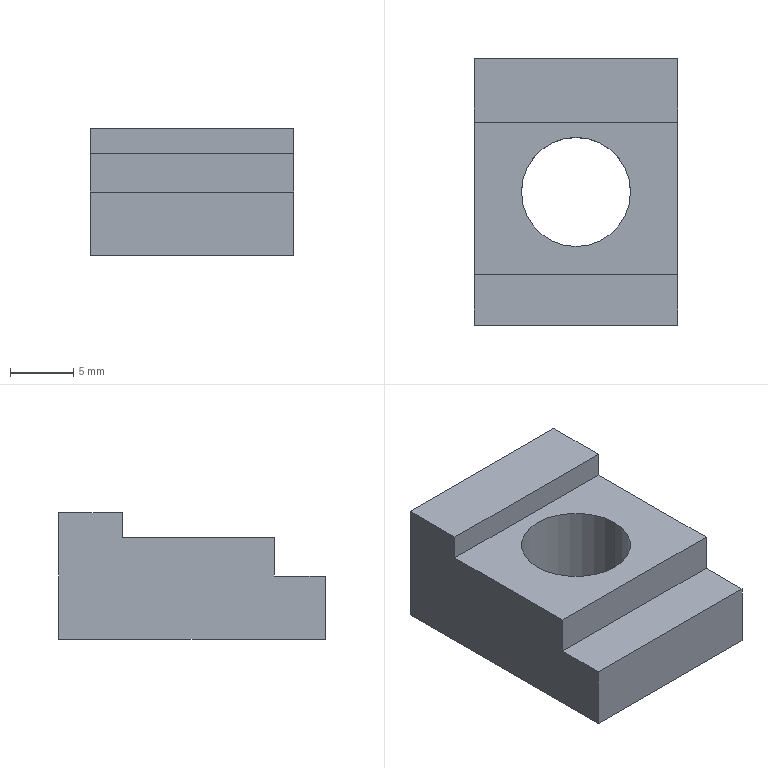Part | STEP file | 1_id1346_x_t | 1 solid | 12 faces | box 16 x 21 x 10 mm | volume 2191 mm3 | plane 10 | cylinder 2 | commonest cylinder face diameters 8.6 x2
STEP:
#1=CARTESIAN_POINT('',(0.,0.,0.));
#2=DIRECTION('',(0.,0.,1.));
#3=DIRECTION('',(1.,0.,0.));
#4=AXIS2_PLACEMENT_3D('',#1,#2,#3);
#5=CARTESIAN_POINT('',(954.138,544.1,90.11));
#6=VERTEX_POINT('',#5);
#7=CARTESIAN_POINT('',(938.138,544.1,90.11));
#8=VERTEX_POINT('',#7);
#9=CARTESIAN_POINT('',(954.138,544.1,90.11));
#10=DIRECTION('',(-1.,0.,0.));
#11=VECTOR('',#10,1.);
#12=LINE('',#9,#11);
#13=CARTESIAN_POINT('',(954.138,544.1,90.11));
#14=DIRECTION('',(0.,0.,-1.));
#15=DIRECTION('',(0.766,-0.6428,0.));
#16=AXIS2_PLACEMENT_3D('',#13,#14,#15);
#17=PLANE('',#16);
#18=CARTESIAN_POINT('',(0.,0.));
#19=DIRECTION('',(-0.766,0.6428));
#20=VECTOR('',#19,1.);
#21=LINE('',#18,#20);
#22=(GEOMETRIC_REPRESENTATION_CONTEXT(2)PARAMETRIC_REPRESENTATION_CONTEXT()REPRESENTATION_CONTEXT('',''));
#23=DEFINITIONAL_REPRESENTATION('',(#21),#22);
#24=PCURVE('',#17,#23);
#25=CARTESIAN_POINT('',(954.138,544.1,85.11));
#26=DIRECTION('',(0.,1.,0.));
#27=DIRECTION('',(0.,0.,1.));
#28=AXIS2_PLACEMENT_3D('',#25,#26,#27);
#29=PLANE('',#28);
#30=CARTESIAN_POINT('',(5.,0.));
#31=DIRECTION('',(0.,-1.));
#32=VECTOR('',#31,1.);
#33=LINE('',#30,#32);
#34=(GEOMETRIC_REPRESENTATION_CONTEXT(2)PARAMETRIC_REPRESENTATION_CONTEXT()REPRESENTATION_CONTEXT('',''));
#35=DEFINITIONAL_REPRESENTATION('',(#33),#34);
#36=PCURVE('',#29,#35);
#37=SURFACE_CURVE('',#12,(#24,#36),.PCURVE_S1.);
#38=EDGE_CURVE('',#6,#8,#37,.T.);
#39=ORIENTED_EDGE('',*,*,#38,.T.);
#40=CARTESIAN_POINT('',(938.138,539.1,90.11));
#41=VERTEX_POINT('',#40);
#42=CARTESIAN_POINT('',(938.138,544.1,90.11));
#43=DIRECTION('',(0.,-1.,0.));
#44=VECTOR('',#43,1.);
#45=LINE('',#42,#44);
#46=CARTESIAN_POINT('',(-12.257,10.285));
#47=DIRECTION('',(0.6428,0.766));
#48=VECTOR('',#47,1.);
#49=LINE('',#46,#48);
#50=(GEOMETRIC_REPRESENTATION_CONTEXT(2)PARAMETRIC_REPRESENTATION_CONTEXT()REPRESENTATION_CONTEXT('',''));
#51=DEFINITIONAL_REPRESENTATION('',(#49),#50);
#52=PCURVE('',#17,#51);
#53=CARTESIAN_POINT('',(938.138,544.1,85.11));
#54=DIRECTION('',(-1.,0.,0.));
#55=DIRECTION('',(0.,1.,0.));
#56=AXIS2_PLACEMENT_3D('',#53,#54,#55);
#57=PLANE('',#56);
#58=CARTESIAN_POINT('',(0.,-5.));
#59=DIRECTION('',(-1.,0.));
#60=VECTOR('',#59,1.);
#61=LINE('',#58,#60);
#62=(GEOMETRIC_REPRESENTATION_CONTEXT(2)PARAMETRIC_REPRESENTATION_CONTEXT()REPRESENTATION_CONTEXT('',''));
#63=DEFINITIONAL_REPRESENTATION('',(#61),#62);
#64=PCURVE('',#57,#63);
#65=SURFACE_CURVE('',#45,(#52,#64),.PCURVE_S1.);
#66=EDGE_CURVE('',#8,#41,#65,.T.);
#67=ORIENTED_EDGE('',*,*,#66,.T.);
#68=CARTESIAN_POINT('',(954.138,539.1,90.11));
#69=VERTEX_POINT('',#68);
#70=CARTESIAN_POINT('',(938.138,539.1,90.11));
#71=DIRECTION('',(1.,0.,0.));
#72=VECTOR('',#71,1.);
#73=LINE('',#70,#72);
#74=CARTESIAN_POINT('',(-9.043,14.115));
#75=DIRECTION('',(0.766,-0.6428));
#76=VECTOR('',#75,1.);
#77=LINE('',#74,#76);
#78=(GEOMETRIC_REPRESENTATION_CONTEXT(2)PARAMETRIC_REPRESENTATION_CONTEXT()REPRESENTATION_CONTEXT('',''));
#79=DEFINITIONAL_REPRESENTATION('',(#77),#78);
#80=PCURVE('',#17,#79);
#81=CARTESIAN_POINT('',(938.138,539.1,91.11));
#82=DIRECTION('',(0.,-1.,0.));
#83=DIRECTION('',(0.,0.,-1.));
#84=AXIS2_PLACEMENT_3D('',#81,#82,#83);
#85=PLANE('',#84);
#86=CARTESIAN_POINT('',(1.,0.));
#87=DIRECTION('',(0.,1.));
#88=VECTOR('',#87,1.);
#89=LINE('',#86,#88);
#90=(GEOMETRIC_REPRESENTATION_CONTEXT(2)PARAMETRIC_REPRESENTATION_CONTEXT()REPRESENTATION_CONTEXT('',''));
#91=DEFINITIONAL_REPRESENTATION('',(#89),#90);
#92=PCURVE('',#85,#91);
#93=SURFACE_CURVE('',#73,(#80,#92),.PCURVE_S1.);
#94=EDGE_CURVE('',#41,#69,#93,.T.);
#95=ORIENTED_EDGE('',*,*,#94,.T.);
#96=CARTESIAN_POINT('',(954.138,539.1,90.11));
#97=DIRECTION('',(0.,1.,0.));
#98=VECTOR('',#97,1.);
#99=LINE('',#96,#98);
#100=CARTESIAN_POINT('',(3.214,3.83));
#101=DIRECTION('',(-0.6428,-0.766));
#102=VECTOR('',#101,1.);
#103=LINE('',#100,#102);
#104=(GEOMETRIC_REPRESENTATION_CONTEXT(2)PARAMETRIC_REPRESENTATION_CONTEXT()REPRESENTATION_CONTEXT('',''));
#105=DEFINITIONAL_REPRESENTATION('',(#103),#104);
#106=PCURVE('',#17,#105);
#107=CARTESIAN_POINT('',(954.138,523.1,85.11));
#108=DIRECTION('',(1.,0.,0.));
#109=DIRECTION('',(0.,0.,1.));
#110=AXIS2_PLACEMENT_3D('',#107,#108,#109);
#111=PLANE('',#110);
#112=CARTESIAN_POINT('',(5.,-16.));
#113=DIRECTION('',(0.,-1.));
#114=VECTOR('',#113,1.);
#115=LINE('',#112,#114);
#116=(GEOMETRIC_REPRESENTATION_CONTEXT(2)PARAMETRIC_REPRESENTATION_CONTEXT()REPRESENTATION_CONTEXT('',''));
#117=DEFINITIONAL_REPRESENTATION('',(#115),#116);
#118=PCURVE('',#111,#117);
#119=SURFACE_CURVE('',#99,(#106,#118),.PCURVE_S1.);
#120=EDGE_CURVE('',#69,#6,#119,.T.);
#121=ORIENTED_EDGE('',*,*,#120,.T.);
#122=EDGE_LOOP('',(#39,#67,#95,#121));
#123=FACE_BOUND('',#122,.T.);
#124=ADVANCED_FACE('',(#123),#17,.F.);
#125=CARTESIAN_POINT('',(954.138,527.1,85.11));
#126=VERTEX_POINT('',#125);
#127=CARTESIAN_POINT('',(954.138,527.1,88.11));
#128=VERTEX_POINT('',#127);
#129=CARTESIAN_POINT('',(954.138,527.1,85.11));
#130=DIRECTION('',(0.,0.,1.));
#131=VECTOR('',#130,1.);
#132=LINE('',#129,#131);
#133=CARTESIAN_POINT('',(0.,-4.));
#134=DIRECTION('',(1.,0.));
#135=VECTOR('',#134,1.);
#136=LINE('',#133,#135);
#137=(GEOMETRIC_REPRESENTATION_CONTEXT(2)PARAMETRIC_REPRESENTATION_CONTEXT()REPRESENTATION_CONTEXT('',''));
#138=DEFINITIONAL_REPRESENTATION('',(#136),#137);
#139=PCURVE('',#111,#138);
#140=CARTESIAN_POINT('',(938.138,527.1,88.11));
#141=DIRECTION('',(0.,-1.,0.));
#142=DIRECTION('',(0.,0.,-1.));
#143=AXIS2_PLACEMENT_3D('',#140,#141,#142);
#144=PLANE('',#143);
#145=CARTESIAN_POINT('',(3.,16.));
#146=DIRECTION('',(-1.,0.));
#147=VECTOR('',#146,1.);
#148=LINE('',#145,#147);
#149=(GEOMETRIC_REPRESENTATION_CONTEXT(2)PARAMETRIC_REPRESENTATION_CONTEXT()REPRESENTATION_CONTEXT('',''));
#150=DEFINITIONAL_REPRESENTATION('',(#148),#149);
#151=PCURVE('',#144,#150);
#152=SURFACE_CURVE('',#132,(#139,#151),.PCURVE_S1.);
#153=EDGE_CURVE('',#126,#128,#152,.T.);
#154=ORIENTED_EDGE('',*,*,#153,.F.);
#155=CARTESIAN_POINT('',(954.138,523.1,85.11));
#156=VERTEX_POINT('',#155);
#157=CARTESIAN_POINT('',(954.138,523.1,85.11));
#158=DIRECTION('',(0.,1.,0.));
#159=VECTOR('',#158,1.);
#160=LINE('',#157,#159);
#161=CARTESIAN_POINT('',(0.,0.));
#162=DIRECTION('',(0.,-1.));
#163=VECTOR('',#162,1.);
#164=LINE('',#161,#163);
#165=(GEOMETRIC_REPRESENTATION_CONTEXT(2)PARAMETRIC_REPRESENTATION_CONTEXT()REPRESENTATION_CONTEXT('',''));
#166=DEFINITIONAL_REPRESENTATION('',(#164),#165);
#167=PCURVE('',#111,#166);
#168=CARTESIAN_POINT('',(938.138,523.1,85.11));
#169=DIRECTION('',(0.,0.,-1.));
#170=DIRECTION('',(0.766,-0.6428,0.));
#171=AXIS2_PLACEMENT_3D('',#168,#169,#170);
#172=PLANE('',#171);
#173=CARTESIAN_POINT('',(12.257,-10.285));
#174=DIRECTION('',(-0.6428,-0.766));
#175=VECTOR('',#174,1.);
#176=LINE('',#173,#175);
#177=(GEOMETRIC_REPRESENTATION_CONTEXT(2)PARAMETRIC_REPRESENTATION_CONTEXT()REPRESENTATION_CONTEXT('',''));
#178=DEFINITIONAL_REPRESENTATION('',(#176),#177);
#179=PCURVE('',#172,#178);
#180=SURFACE_CURVE('',#160,(#167,#179),.PCURVE_S1.);
#181=EDGE_CURVE('',#156,#126,#180,.T.);
#182=ORIENTED_EDGE('',*,*,#181,.F.);
#183=CARTESIAN_POINT('',(954.138,523.1,80.11));
#184=VERTEX_POINT('',#183);
#185=CARTESIAN_POINT('',(954.138,523.1,80.11));
#186=DIRECTION('',(0.,0.,1.));
#187=VECTOR('',#186,1.);
#188=LINE('',#185,#187);
#189=CARTESIAN_POINT('',(-5.,0.));
#190=DIRECTION('',(1.,0.));
#191=VECTOR('',#190,1.);
#192=LINE('',#189,#191);
#193=(GEOMETRIC_REPRESENTATION_CONTEXT(2)PARAMETRIC_REPRESENTATION_CONTEXT()REPRESENTATION_CONTEXT('',''));
#194=DEFINITIONAL_REPRESENTATION('',(#192),#193);
#195=PCURVE('',#111,#194);
#196=CARTESIAN_POINT('',(938.138,523.1,85.11));
#197=DIRECTION('',(0.,-1.,0.));
#198=DIRECTION('',(0.,0.,-1.));
#199=AXIS2_PLACEMENT_3D('',#196,#197,#198);
#200=PLANE('',#199);
#201=CARTESIAN_POINT('',(5.,16.));
#202=DIRECTION('',(-1.,0.));
#203=VECTOR('',#202,1.);
#204=LINE('',#201,#203);
#205=(GEOMETRIC_REPRESENTATION_CONTEXT(2)PARAMETRIC_REPRESENTATION_CONTEXT()REPRESENTATION_CONTEXT('',''));
#206=DEFINITIONAL_REPRESENTATION('',(#204),#205);
#207=PCURVE('',#200,#206);
#208=SURFACE_CURVE('',#188,(#195,#207),.PCURVE_S1.);
#209=EDGE_CURVE('',#184,#156,#208,.T.);
#210=ORIENTED_EDGE('',*,*,#209,.F.);
#211=CARTESIAN_POINT('',(954.138,544.1,80.11));
#212=VERTEX_POINT('',#211);
#213=CARTESIAN_POINT('',(954.138,544.1,80.11));
#214=DIRECTION('',(0.,-1.,0.));
#215=VECTOR('',#214,1.);
#216=LINE('',#213,#215);
#217=CARTESIAN_POINT('',(-5.,-21.));
#218=DIRECTION('',(0.,1.));
#219=VECTOR('',#218,1.);
#220=LINE('',#217,#219);
#221=(GEOMETRIC_REPRESENTATION_CONTEXT(2)PARAMETRIC_REPRESENTATION_CONTEXT()REPRESENTATION_CONTEXT('',''));
#222=DEFINITIONAL_REPRESENTATION('',(#220),#221);
#223=PCURVE('',#111,#222);
#224=CARTESIAN_POINT('',(938.138,523.1,80.11));
#225=DIRECTION('',(0.,0.,-1.));
#226=DIRECTION('',(0.766,-0.6428,0.));
#227=AXIS2_PLACEMENT_3D('',#224,#225,#226);
#228=PLANE('',#227);
#229=CARTESIAN_POINT('',(-1.242,-26.372));
#230=DIRECTION('',(0.6428,0.766));
#231=VECTOR('',#230,1.);
#232=LINE('',#229,#231);
#233=(GEOMETRIC_REPRESENTATION_CONTEXT(2)PARAMETRIC_REPRESENTATION_CONTEXT()REPRESENTATION_CONTEXT('',''));
#234=DEFINITIONAL_REPRESENTATION('',(#232),#233);
#235=PCURVE('',#228,#234);
#236=SURFACE_CURVE('',#216,(#223,#235),.PCURVE_S1.);
#237=EDGE_CURVE('',#212,#184,#236,.T.);
#238=ORIENTED_EDGE('',*,*,#237,.F.);
#239=CARTESIAN_POINT('',(954.138,544.1,80.11));
#240=DIRECTION('',(0.,0.,1.));
#241=VECTOR('',#240,1.);
#242=LINE('',#239,#241);
#243=CARTESIAN_POINT('',(-5.,-21.));
#244=DIRECTION('',(1.,0.));
#245=VECTOR('',#244,1.);
#246=LINE('',#243,#245);
#247=(GEOMETRIC_REPRESENTATION_CONTEXT(2)PARAMETRIC_REPRESENTATION_CONTEXT()REPRESENTATION_CONTEXT('',''));
#248=DEFINITIONAL_REPRESENTATION('',(#246),#247);
#249=PCURVE('',#111,#248);
#250=CARTESIAN_POINT('',(-5.,0.));
#251=DIRECTION('',(1.,0.));
#252=VECTOR('',#251,1.);
#253=LINE('',#250,#252);
#254=(GEOMETRIC_REPRESENTATION_CONTEXT(2)PARAMETRIC_REPRESENTATION_CONTEXT()REPRESENTATION_CONTEXT('',''));
#255=DEFINITIONAL_REPRESENTATION('',(#253),#254);
#256=PCURVE('',#29,#255);
#257=SURFACE_CURVE('',#242,(#249,#256),.PCURVE_S1.);
#258=EDGE_CURVE('',#212,#6,#257,.T.);
#259=ORIENTED_EDGE('',*,*,#258,.T.);
#260=ORIENTED_EDGE('',*,*,#120,.F.);
#261=CARTESIAN_POINT('',(954.138,539.1,88.11));
#262=VERTEX_POINT('',#261);
#263=CARTESIAN_POINT('',(954.138,539.1,88.11));
#264=DIRECTION('',(0.,0.,1.));
#265=VECTOR('',#264,1.);
#266=LINE('',#263,#265);
#267=CARTESIAN_POINT('',(3.,-16.));
#268=DIRECTION('',(1.,0.));
#269=VECTOR('',#268,1.);
#270=LINE('',#267,#269);
#271=(GEOMETRIC_REPRESENTATION_CONTEXT(2)PARAMETRIC_REPRESENTATION_CONTEXT()REPRESENTATION_CONTEXT('',''));
#272=DEFINITIONAL_REPRESENTATION('',(#270),#271);
#273=PCURVE('',#111,#272);
#274=CARTESIAN_POINT('',(3.,16.));
#275=DIRECTION('',(-1.,0.));
#276=VECTOR('',#275,1.);
#277=LINE('',#274,#276);
#278=(GEOMETRIC_REPRESENTATION_CONTEXT(2)PARAMETRIC_REPRESENTATION_CONTEXT()REPRESENTATION_CONTEXT('',''));
#279=DEFINITIONAL_REPRESENTATION('',(#277),#278);
#280=PCURVE('',#85,#279);
#281=SURFACE_CURVE('',#266,(#273,#280),.PCURVE_S1.);
#282=EDGE_CURVE('',#262,#69,#281,.T.);
#283=ORIENTED_EDGE('',*,*,#282,.F.);
#284=CARTESIAN_POINT('',(954.138,527.1,88.11));
#285=DIRECTION('',(0.,1.,0.));
#286=VECTOR('',#285,1.);
#287=LINE('',#284,#286);
#288=CARTESIAN_POINT('',(3.,-4.));
#289=DIRECTION('',(0.,-1.));
#290=VECTOR('',#289,1.);
#291=LINE('',#288,#290);
#292=(GEOMETRIC_REPRESENTATION_CONTEXT(2)PARAMETRIC_REPRESENTATION_CONTEXT()REPRESENTATION_CONTEXT('',''));
#293=DEFINITIONAL_REPRESENTATION('',(#291),#292);
#294=PCURVE('',#111,#293);
#295=CARTESIAN_POINT('',(954.138,544.1,88.11));
#296=DIRECTION('',(0.,0.,-1.));
#297=DIRECTION('',(0.766,-0.6428,0.));
#298=AXIS2_PLACEMENT_3D('',#295,#296,#297);
#299=PLANE('',#298);
#300=CARTESIAN_POINT('',(10.927,13.023));
#301=DIRECTION('',(-0.6428,-0.766));
#302=VECTOR('',#301,1.);
#303=LINE('',#300,#302);
#304=(GEOMETRIC_REPRESENTATION_CONTEXT(2)PARAMETRIC_REPRESENTATION_CONTEXT()REPRESENTATION_CONTEXT('',''));
#305=DEFINITIONAL_REPRESENTATION('',(#303),#304);
#306=PCURVE('',#299,#305);
#307=SURFACE_CURVE('',#287,(#294,#306),.PCURVE_S1.);
#308=EDGE_CURVE('',#128,#262,#307,.T.);
#309=ORIENTED_EDGE('',*,*,#308,.F.);
#310=EDGE_LOOP('',(#154,#182,#210,#238,#259,#260,#283,#309));
#311=FACE_BOUND('',#310,.T.);
#312=ADVANCED_FACE('',(#311),#111,.T.);
#313=CARTESIAN_POINT('',(938.138,527.1,88.11));
#314=VERTEX_POINT('',#313);
#315=CARTESIAN_POINT('',(938.138,527.1,88.11));
#316=DIRECTION('',(1.,0.,0.));
#317=VECTOR('',#316,1.);
#318=LINE('',#315,#317);
#319=CARTESIAN_POINT('',(-1.329,23.307));
#320=DIRECTION('',(0.766,-0.6428));
#321=VECTOR('',#320,1.);
#322=LINE('',#319,#321);
#323=(GEOMETRIC_REPRESENTATION_CONTEXT(2)PARAMETRIC_REPRESENTATION_CONTEXT()REPRESENTATION_CONTEXT('',''));
#324=DEFINITIONAL_REPRESENTATION('',(#322),#323);
#325=PCURVE('',#299,#324);
#326=CARTESIAN_POINT('',(0.,0.));
#327=DIRECTION('',(0.,1.));
#328=VECTOR('',#327,1.);
#329=LINE('',#326,#328);
#330=(GEOMETRIC_REPRESENTATION_CONTEXT(2)PARAMETRIC_REPRESENTATION_CONTEXT()REPRESENTATION_CONTEXT('',''));
#331=DEFINITIONAL_REPRESENTATION('',(#329),#330);
#332=PCURVE('',#144,#331);
#333=SURFACE_CURVE('',#318,(#325,#332),.PCURVE_S1.);
#334=EDGE_CURVE('',#314,#128,#333,.T.);
#335=ORIENTED_EDGE('',*,*,#334,.T.);
#336=ORIENTED_EDGE('',*,*,#308,.T.);
#337=CARTESIAN_POINT('',(938.138,539.1,88.11));
#338=VERTEX_POINT('',#337);
#339=CARTESIAN_POINT('',(954.138,539.1,88.11));
#340=DIRECTION('',(-1.,0.,0.));
#341=VECTOR('',#340,1.);
#342=LINE('',#339,#341);
#343=CARTESIAN_POINT('',(3.214,3.83));
#344=DIRECTION('',(-0.766,0.6428));
#345=VECTOR('',#344,1.);
#346=LINE('',#343,#345);
#347=(GEOMETRIC_REPRESENTATION_CONTEXT(2)PARAMETRIC_REPRESENTATION_CONTEXT()REPRESENTATION_CONTEXT('',''));
#348=DEFINITIONAL_REPRESENTATION('',(#346),#347);
#349=PCURVE('',#299,#348);
#350=CARTESIAN_POINT('',(3.,16.));
#351=DIRECTION('',(0.,-1.));
#352=VECTOR('',#351,1.);
#353=LINE('',#350,#352);
#354=(GEOMETRIC_REPRESENTATION_CONTEXT(2)PARAMETRIC_REPRESENTATION_CONTEXT()REPRESENTATION_CONTEXT('',''));
#355=DEFINITIONAL_REPRESENTATION('',(#353),#354);
#356=PCURVE('',#85,#355);
#357=SURFACE_CURVE('',#342,(#349,#356),.PCURVE_S1.);
#358=EDGE_CURVE('',#262,#338,#357,.T.);
#359=ORIENTED_EDGE('',*,*,#358,.T.);
#360=CARTESIAN_POINT('',(938.138,539.1,88.11));
#361=DIRECTION('',(0.,-1.,0.));
#362=VECTOR('',#361,1.);
#363=LINE('',#360,#362);
#364=CARTESIAN_POINT('',(-9.043,14.115));
#365=DIRECTION('',(0.6428,0.766));
#366=VECTOR('',#365,1.);
#367=LINE('',#364,#366);
#368=(GEOMETRIC_REPRESENTATION_CONTEXT(2)PARAMETRIC_REPRESENTATION_CONTEXT()REPRESENTATION_CONTEXT('',''));
#369=DEFINITIONAL_REPRESENTATION('',(#367),#368);
#370=PCURVE('',#299,#369);
#371=CARTESIAN_POINT('',(-5.,-3.));
#372=DIRECTION('',(-1.,0.));
#373=VECTOR('',#372,1.);
#374=LINE('',#371,#373);
#375=(GEOMETRIC_REPRESENTATION_CONTEXT(2)PARAMETRIC_REPRESENTATION_CONTEXT()REPRESENTATION_CONTEXT('',''));
#376=DEFINITIONAL_REPRESENTATION('',(#374),#375);
#377=PCURVE('',#57,#376);
#378=SURFACE_CURVE('',#363,(#370,#377),.PCURVE_S1.);
#379=EDGE_CURVE('',#338,#314,#378,.T.);
#380=ORIENTED_EDGE('',*,*,#379,.T.);
#381=EDGE_LOOP('',(#335,#336,#359,#380));
#382=FACE_BOUND('',#381,.T.);
#383=CARTESIAN_POINT('',(941.838,533.6,88.11));
#384=VERTEX_POINT('',#383);
#385=CARTESIAN_POINT('',(950.438,533.6,88.11));
#386=VERTEX_POINT('',#385);
#387=CARTESIAN_POINT('',(946.138,533.6,88.11));
#388=DIRECTION('',(0.,0.,-1.));
#389=DIRECTION('',(-1.,0.,0.));
#390=AXIS2_PLACEMENT_3D('',#387,#388,#389);
#391=CIRCLE('',#390,4.3);
#392=CARTESIAN_POINT('',(0.6209,13.186));
#393=DIRECTION('',(-0.766,0.6428));
#394=AXIS2_PLACEMENT_2D('',#392,#393);
#395=CIRCLE('',#394,4.3);
#396=(GEOMETRIC_REPRESENTATION_CONTEXT(2)PARAMETRIC_REPRESENTATION_CONTEXT()REPRESENTATION_CONTEXT('',''));
#397=DEFINITIONAL_REPRESENTATION('',(#395),#396);
#398=PCURVE('',#299,#397);
#399=CARTESIAN_POINT('',(946.138,533.6,108.03));
#400=DIRECTION('',(0.,0.,1.));
#401=DIRECTION('',(1.,0.,0.));
#402=AXIS2_PLACEMENT_3D('',#399,#400,#401);
#403=CYLINDRICAL_SURFACE('',#402,4.3);
#404=CARTESIAN_POINT('',(3.142,-19.92));
#405=DIRECTION('',(-1.,0.));
#406=VECTOR('',#405,1.);
#407=LINE('',#404,#406);
#408=(GEOMETRIC_REPRESENTATION_CONTEXT(2)PARAMETRIC_REPRESENTATION_CONTEXT()REPRESENTATION_CONTEXT('',''));
#409=DEFINITIONAL_REPRESENTATION('',(#407),#408);
#410=PCURVE('',#403,#409);
#411=SURFACE_CURVE('',#391,(#398,#410),.PCURVE_S1.);
#412=EDGE_CURVE('',#384,#386,#411,.T.);
#413=ORIENTED_EDGE('',*,*,#412,.T.);
#414=CARTESIAN_POINT('',(946.138,533.6,88.11));
#415=DIRECTION('',(0.,0.,-1.));
#416=DIRECTION('',(1.,0.,0.));
#417=AXIS2_PLACEMENT_3D('',#414,#415,#416);
#418=CIRCLE('',#417,4.3);
#419=CARTESIAN_POINT('',(0.6209,13.186));
#420=DIRECTION('',(0.766,-0.6428));
#421=AXIS2_PLACEMENT_2D('',#419,#420);
#422=CIRCLE('',#421,4.3);
#423=(GEOMETRIC_REPRESENTATION_CONTEXT(2)PARAMETRIC_REPRESENTATION_CONTEXT()REPRESENTATION_CONTEXT('',''));
#424=DEFINITIONAL_REPRESENTATION('',(#422),#423);
#425=PCURVE('',#299,#424);
#426=CARTESIAN_POINT('',(946.138,533.6,108.03));
#427=DIRECTION('',(0.,0.,1.));
#428=DIRECTION('',(1.,0.,0.));
#429=AXIS2_PLACEMENT_3D('',#426,#427,#428);
#430=CYLINDRICAL_SURFACE('',#429,4.3);
#431=CARTESIAN_POINT('',(6.283,-19.92));
#432=DIRECTION('',(-1.,0.));
#433=VECTOR('',#432,1.);
#434=LINE('',#431,#433);
#435=(GEOMETRIC_REPRESENTATION_CONTEXT(2)PARAMETRIC_REPRESENTATION_CONTEXT()REPRESENTATION_CONTEXT('',''));
#436=DEFINITIONAL_REPRESENTATION('',(#434),#435);
#437=PCURVE('',#430,#436);
#438=SURFACE_CURVE('',#418,(#425,#437),.PCURVE_S1.);
#439=EDGE_CURVE('',#386,#384,#438,.T.);
#440=ORIENTED_EDGE('',*,*,#439,.T.);
#441=EDGE_LOOP('',(#413,#440));
#442=FACE_BOUND('',#441,.T.);
#443=ADVANCED_FACE('',(#382,#442),#299,.F.);
#444=CARTESIAN_POINT('',(938.138,527.1,85.11));
#445=VERTEX_POINT('',#444);
#446=CARTESIAN_POINT('',(938.138,523.1,85.11));
#447=VERTEX_POINT('',#446);
#448=CARTESIAN_POINT('',(938.138,527.1,85.11));
#449=DIRECTION('',(0.,-1.,0.));
#450=VECTOR('',#449,1.);
#451=LINE('',#448,#450);
#452=CARTESIAN_POINT('',(-17.,0.));
#453=DIRECTION('',(-1.,0.));
#454=VECTOR('',#453,1.);
#455=LINE('',#452,#454);
#456=(GEOMETRIC_REPRESENTATION_CONTEXT(2)PARAMETRIC_REPRESENTATION_CONTEXT()REPRESENTATION_CONTEXT('',''));
#457=DEFINITIONAL_REPRESENTATION('',(#455),#456);
#458=PCURVE('',#57,#457);
#459=CARTESIAN_POINT('',(-2.571,-3.064));
#460=DIRECTION('',(0.6428,0.766));
#461=VECTOR('',#460,1.);
#462=LINE('',#459,#461);
#463=(GEOMETRIC_REPRESENTATION_CONTEXT(2)PARAMETRIC_REPRESENTATION_CONTEXT()REPRESENTATION_CONTEXT('',''));
#464=DEFINITIONAL_REPRESENTATION('',(#462),#463);
#465=PCURVE('',#172,#464);
#466=SURFACE_CURVE('',#451,(#458,#465),.PCURVE_S1.);
#467=EDGE_CURVE('',#445,#447,#466,.T.);
#468=ORIENTED_EDGE('',*,*,#467,.F.);
#469=CARTESIAN_POINT('',(938.138,527.1,85.11));
#470=DIRECTION('',(0.,0.,1.));
#471=VECTOR('',#470,1.);
#472=LINE('',#469,#471);
#473=CARTESIAN_POINT('',(-17.,0.));
#474=DIRECTION('',(0.,-1.));
#475=VECTOR('',#474,1.);
#476=LINE('',#473,#475);
#477=(GEOMETRIC_REPRESENTATION_CONTEXT(2)PARAMETRIC_REPRESENTATION_CONTEXT()REPRESENTATION_CONTEXT('',''));
#478=DEFINITIONAL_REPRESENTATION('',(#476),#477);
#479=PCURVE('',#57,#478);
#480=CARTESIAN_POINT('',(3.,0.));
#481=DIRECTION('',(-1.,0.));
#482=VECTOR('',#481,1.);
#483=LINE('',#480,#482);
#484=(GEOMETRIC_REPRESENTATION_CONTEXT(2)PARAMETRIC_REPRESENTATION_CONTEXT()REPRESENTATION_CONTEXT('',''));
#485=DEFINITIONAL_REPRESENTATION('',(#483),#484);
#486=PCURVE('',#144,#485);
#487=SURFACE_CURVE('',#472,(#479,#486),.PCURVE_S1.);
#488=EDGE_CURVE('',#445,#314,#487,.T.);
#489=ORIENTED_EDGE('',*,*,#488,.T.);
#490=ORIENTED_EDGE('',*,*,#379,.F.);
#491=CARTESIAN_POINT('',(938.138,539.1,88.11));
#492=DIRECTION('',(0.,0.,1.));
#493=VECTOR('',#492,1.);
#494=LINE('',#491,#493);
#495=CARTESIAN_POINT('',(-5.,-3.));
#496=DIRECTION('',(0.,-1.));
#497=VECTOR('',#496,1.);
#498=LINE('',#495,#497);
#499=(GEOMETRIC_REPRESENTATION_CONTEXT(2)PARAMETRIC_REPRESENTATION_CONTEXT()REPRESENTATION_CONTEXT('',''));
#500=DEFINITIONAL_REPRESENTATION('',(#498),#499);
#501=PCURVE('',#57,#500);
#502=CARTESIAN_POINT('',(3.,0.));
#503=DIRECTION('',(-1.,0.));
#504=VECTOR('',#503,1.);
#505=LINE('',#502,#504);
#506=(GEOMETRIC_REPRESENTATION_CONTEXT(2)PARAMETRIC_REPRESENTATION_CONTEXT()REPRESENTATION_CONTEXT('',''));
#507=DEFINITIONAL_REPRESENTATION('',(#505),#506);
#508=PCURVE('',#85,#507);
#509=SURFACE_CURVE('',#494,(#501,#508),.PCURVE_S1.);
#510=EDGE_CURVE('',#338,#41,#509,.T.);
#511=ORIENTED_EDGE('',*,*,#510,.T.);
#512=ORIENTED_EDGE('',*,*,#66,.F.);
#513=CARTESIAN_POINT('',(938.138,544.1,80.11));
#514=VERTEX_POINT('',#513);
#515=CARTESIAN_POINT('',(938.138,544.1,80.11));
#516=DIRECTION('',(0.,0.,1.));
#517=VECTOR('',#516,1.);
#518=LINE('',#515,#517);
#519=CARTESIAN_POINT('',(0.,5.));
#520=DIRECTION('',(0.,-1.));
#521=VECTOR('',#520,1.);
#522=LINE('',#519,#521);
#523=(GEOMETRIC_REPRESENTATION_CONTEXT(2)PARAMETRIC_REPRESENTATION_CONTEXT()REPRESENTATION_CONTEXT('',''));
#524=DEFINITIONAL_REPRESENTATION('',(#522),#523);
#525=PCURVE('',#57,#524);
#526=CARTESIAN_POINT('',(-5.,-16.));
#527=DIRECTION('',(1.,0.));
#528=VECTOR('',#527,1.);
#529=LINE('',#526,#528);
#530=(GEOMETRIC_REPRESENTATION_CONTEXT(2)PARAMETRIC_REPRESENTATION_CONTEXT()REPRESENTATION_CONTEXT('',''));
#531=DEFINITIONAL_REPRESENTATION('',(#529),#530);
#532=PCURVE('',#29,#531);
#533=SURFACE_CURVE('',#518,(#525,#532),.PCURVE_S1.);
#534=EDGE_CURVE('',#514,#8,#533,.T.);
#535=ORIENTED_EDGE('',*,*,#534,.F.);
#536=CARTESIAN_POINT('',(938.138,523.1,80.11));
#537=VERTEX_POINT('',#536);
#538=CARTESIAN_POINT('',(938.138,523.1,80.11));
#539=DIRECTION('',(0.,1.,0.));
#540=VECTOR('',#539,1.);
#541=LINE('',#538,#540);
#542=CARTESIAN_POINT('',(-21.,5.));
#543=DIRECTION('',(1.,0.));
#544=VECTOR('',#543,1.);
#545=LINE('',#542,#544);
#546=(GEOMETRIC_REPRESENTATION_CONTEXT(2)PARAMETRIC_REPRESENTATION_CONTEXT()REPRESENTATION_CONTEXT('',''));
#547=DEFINITIONAL_REPRESENTATION('',(#545),#546);
#548=PCURVE('',#57,#547);
#549=CARTESIAN_POINT('',(0.,0.));
#550=DIRECTION('',(-0.6428,-0.766));
#551=VECTOR('',#550,1.);
#552=LINE('',#549,#551);
#553=(GEOMETRIC_REPRESENTATION_CONTEXT(2)PARAMETRIC_REPRESENTATION_CONTEXT()REPRESENTATION_CONTEXT('',''));
#554=DEFINITIONAL_REPRESENTATION('',(#552),#553);
#555=PCURVE('',#228,#554);
#556=SURFACE_CURVE('',#541,(#548,#555),.PCURVE_S1.);
#557=EDGE_CURVE('',#537,#514,#556,.T.);
#558=ORIENTED_EDGE('',*,*,#557,.F.);
#559=CARTESIAN_POINT('',(938.138,523.1,80.11));
#560=DIRECTION('',(0.,0.,1.));
#561=VECTOR('',#560,1.);
#562=LINE('',#559,#561);
#563=CARTESIAN_POINT('',(-21.,5.));
#564=DIRECTION('',(0.,-1.));
#565=VECTOR('',#564,1.);
#566=LINE('',#563,#565);
#567=(GEOMETRIC_REPRESENTATION_CONTEXT(2)PARAMETRIC_REPRESENTATION_CONTEXT()REPRESENTATION_CONTEXT('',''));
#568=DEFINITIONAL_REPRESENTATION('',(#566),#567);
#569=PCURVE('',#57,#568);
#570=CARTESIAN_POINT('',(5.,0.));
#571=DIRECTION('',(-1.,0.));
#572=VECTOR('',#571,1.);
#573=LINE('',#570,#572);
#574=(GEOMETRIC_REPRESENTATION_CONTEXT(2)PARAMETRIC_REPRESENTATION_CONTEXT()REPRESENTATION_CONTEXT('',''));
#575=DEFINITIONAL_REPRESENTATION('',(#573),#574);
#576=PCURVE('',#200,#575);
#577=SURFACE_CURVE('',#562,(#569,#576),.PCURVE_S1.);
#578=EDGE_CURVE('',#537,#447,#577,.T.);
#579=ORIENTED_EDGE('',*,*,#578,.T.);
#580=EDGE_LOOP('',(#468,#489,#490,#511,#512,#535,#558,#579));
#581=FACE_BOUND('',#580,.T.);
#582=ADVANCED_FACE('',(#581),#57,.T.);
#583=ORIENTED_EDGE('',*,*,#209,.T.);
#584=CARTESIAN_POINT('',(938.138,523.1,85.11));
#585=DIRECTION('',(1.,0.,0.));
#586=VECTOR('',#585,1.);
#587=LINE('',#584,#586);
#588=CARTESIAN_POINT('',(0.,0.));
#589=DIRECTION('',(0.,1.));
#590=VECTOR('',#589,1.);
#591=LINE('',#588,#590);
#592=(GEOMETRIC_REPRESENTATION_CONTEXT(2)PARAMETRIC_REPRESENTATION_CONTEXT()REPRESENTATION_CONTEXT('',''));
#593=DEFINITIONAL_REPRESENTATION('',(#591),#592);
#594=PCURVE('',#200,#593);
#595=CARTESIAN_POINT('',(0.,0.));
#596=DIRECTION('',(0.766,-0.6428));
#597=VECTOR('',#596,1.);
#598=LINE('',#595,#597);
#599=(GEOMETRIC_REPRESENTATION_CONTEXT(2)PARAMETRIC_REPRESENTATION_CONTEXT()REPRESENTATION_CONTEXT('',''));
#600=DEFINITIONAL_REPRESENTATION('',(#598),#599);
#601=PCURVE('',#172,#600);
#602=SURFACE_CURVE('',#587,(#594,#601),.PCURVE_S1.);
#603=EDGE_CURVE('',#447,#156,#602,.T.);
#604=ORIENTED_EDGE('',*,*,#603,.F.);
#605=ORIENTED_EDGE('',*,*,#578,.F.);
#606=CARTESIAN_POINT('',(954.138,523.1,80.11));
#607=DIRECTION('',(-1.,0.,0.));
#608=VECTOR('',#607,1.);
#609=LINE('',#606,#608);
#610=CARTESIAN_POINT('',(5.,16.));
#611=DIRECTION('',(0.,-1.));
#612=VECTOR('',#611,1.);
#613=LINE('',#610,#612);
#614=(GEOMETRIC_REPRESENTATION_CONTEXT(2)PARAMETRIC_REPRESENTATION_CONTEXT()REPRESENTATION_CONTEXT('',''));
#615=DEFINITIONAL_REPRESENTATION('',(#613),#614);
#616=PCURVE('',#200,#615);
#617=CARTESIAN_POINT('',(12.257,-10.285));
#618=DIRECTION('',(-0.766,0.6428));
#619=VECTOR('',#618,1.);
#620=LINE('',#617,#619);
#621=(GEOMETRIC_REPRESENTATION_CONTEXT(2)PARAMETRIC_REPRESENTATION_CONTEXT()REPRESENTATION_CONTEXT('',''));
#622=DEFINITIONAL_REPRESENTATION('',(#620),#621);
#623=PCURVE('',#228,#622);
#624=SURFACE_CURVE('',#609,(#616,#623),.PCURVE_S1.);
#625=EDGE_CURVE('',#184,#537,#624,.T.);
#626=ORIENTED_EDGE('',*,*,#625,.F.);
#627=EDGE_LOOP('',(#583,#604,#605,#626));
#628=FACE_BOUND('',#627,.T.);
#629=ADVANCED_FACE('',(#628),#200,.T.);
#630=ORIENTED_EDGE('',*,*,#625,.T.);
#631=ORIENTED_EDGE('',*,*,#557,.T.);
#632=CARTESIAN_POINT('',(938.138,544.1,80.11));
#633=DIRECTION('',(1.,0.,0.));
#634=VECTOR('',#633,1.);
#635=LINE('',#632,#634);
#636=CARTESIAN_POINT('',(-13.499,-16.087));
#637=DIRECTION('',(0.766,-0.6428));
#638=VECTOR('',#637,1.);
#639=LINE('',#636,#638);
#640=(GEOMETRIC_REPRESENTATION_CONTEXT(2)PARAMETRIC_REPRESENTATION_CONTEXT()REPRESENTATION_CONTEXT('',''));
#641=DEFINITIONAL_REPRESENTATION('',(#639),#640);
#642=PCURVE('',#228,#641);
#643=CARTESIAN_POINT('',(-5.,-16.));
#644=DIRECTION('',(0.,1.));
#645=VECTOR('',#644,1.);
#646=LINE('',#643,#645);
#647=(GEOMETRIC_REPRESENTATION_CONTEXT(2)PARAMETRIC_REPRESENTATION_CONTEXT()REPRESENTATION_CONTEXT('',''));
#648=DEFINITIONAL_REPRESENTATION('',(#646),#647);
#649=PCURVE('',#29,#648);
#650=SURFACE_CURVE('',#635,(#642,#649),.PCURVE_S1.);
#651=EDGE_CURVE('',#514,#212,#650,.T.);
#652=ORIENTED_EDGE('',*,*,#651,.T.);
#653=ORIENTED_EDGE('',*,*,#237,.T.);
#654=EDGE_LOOP('',(#630,#631,#652,#653));
#655=FACE_BOUND('',#654,.T.);
#656=CARTESIAN_POINT('',(941.838,533.6,80.11));
#657=VERTEX_POINT('',#656);
#658=CARTESIAN_POINT('',(950.438,533.6,80.11));
#659=VERTEX_POINT('',#658);
#660=CARTESIAN_POINT('',(946.138,533.6,80.11));
#661=DIRECTION('',(0.,0.,1.));
#662=DIRECTION('',(-1.,0.,0.));
#663=AXIS2_PLACEMENT_3D('',#660,#661,#662);
#664=CIRCLE('',#663,4.3);
#665=CARTESIAN_POINT('',(-3.915,-10.422));
#666=CARTESIAN_POINT('',(0.8725,-4.716));
#667=CARTESIAN_POINT('',(3.42,-11.715));
#668=CARTESIAN_POINT('',(5.967,-18.714));
#669=CARTESIAN_POINT('',(-1.368,-17.42));
#670=CARTESIAN_POINT('',(-8.702,-16.127));
#671=CARTESIAN_POINT('',(-3.915,-10.422));
#672=(BOUNDED_CURVE()B_SPLINE_CURVE(2,(#665,#666,#667,#668,#669,#670,#671),.UNSPECIFIED.,.T.,.F.)B_SPLINE_CURVE_WITH_KNOTS((1,2,2,2,2,1),(-2.094,0.,2.094,4.189,6.283,8.378),.UNSPECIFIED.)CURVE()GEOMETRIC_REPRESENTATION_ITEM()RATIONAL_B_SPLINE_CURVE((1.,0.5,1.,0.5,1.,0.5,1.))REPRESENTATION_ITEM(''));
#673=(GEOMETRIC_REPRESENTATION_CONTEXT(2)PARAMETRIC_REPRESENTATION_CONTEXT()REPRESENTATION_CONTEXT('',''));
#674=DEFINITIONAL_REPRESENTATION('',(#672),#673);
#675=PCURVE('',#228,#674);
#676=CARTESIAN_POINT('',(3.142,-27.92));
#677=DIRECTION('',(1.,0.));
#678=VECTOR('',#677,1.);
#679=LINE('',#676,#678);
#680=(GEOMETRIC_REPRESENTATION_CONTEXT(2)PARAMETRIC_REPRESENTATION_CONTEXT()REPRESENTATION_CONTEXT('',''));
#681=DEFINITIONAL_REPRESENTATION('',(#679),#680);
#682=PCURVE('',#430,#681);
#683=SURFACE_CURVE('',#664,(#675,#682),.PCURVE_S1.);
#684=EDGE_CURVE('',#657,#659,#683,.T.);
#685=ORIENTED_EDGE('',*,*,#684,.T.);
#686=CARTESIAN_POINT('',(946.138,533.6,80.11));
#687=DIRECTION('',(0.,0.,1.));
#688=DIRECTION('',(1.,0.,0.));
#689=AXIS2_PLACEMENT_3D('',#686,#687,#688);
#690=CIRCLE('',#689,4.3);
#691=CARTESIAN_POINT('',(2.673,-15.95));
#692=CARTESIAN_POINT('',(-2.114,-21.655));
#693=CARTESIAN_POINT('',(-4.662,-14.656));
#694=CARTESIAN_POINT('',(-7.209,-7.658));
#695=CARTESIAN_POINT('',(0.1258,-8.951));
#696=CARTESIAN_POINT('',(7.46,-10.244));
#697=CARTESIAN_POINT('',(2.673,-15.95));
#698=(BOUNDED_CURVE()B_SPLINE_CURVE(2,(#691,#692,#693,#694,#695,#696,#697),.UNSPECIFIED.,.T.,.F.)B_SPLINE_CURVE_WITH_KNOTS((1,2,2,2,2,1),(-2.094,0.,2.094,4.189,6.283,8.378),.UNSPECIFIED.)CURVE()GEOMETRIC_REPRESENTATION_ITEM()RATIONAL_B_SPLINE_CURVE((1.,0.5,1.,0.5,1.,0.5,1.))REPRESENTATION_ITEM(''));
#699=(GEOMETRIC_REPRESENTATION_CONTEXT(2)PARAMETRIC_REPRESENTATION_CONTEXT()REPRESENTATION_CONTEXT('',''));
#700=DEFINITIONAL_REPRESENTATION('',(#698),#699);
#701=PCURVE('',#228,#700);
#702=CARTESIAN_POINT('',(0.,-27.92));
#703=DIRECTION('',(1.,0.));
#704=VECTOR('',#703,1.);
#705=LINE('',#702,#704);
#706=(GEOMETRIC_REPRESENTATION_CONTEXT(2)PARAMETRIC_REPRESENTATION_CONTEXT()REPRESENTATION_CONTEXT('',''));
#707=DEFINITIONAL_REPRESENTATION('',(#705),#706);
#708=PCURVE('',#403,#707);
#709=SURFACE_CURVE('',#690,(#701,#708),.PCURVE_S1.);
#710=EDGE_CURVE('',#659,#657,#709,.T.);
#711=ORIENTED_EDGE('',*,*,#710,.T.);
#712=EDGE_LOOP('',(#685,#711));
#713=FACE_BOUND('',#712,.T.);
#714=ADVANCED_FACE('',(#655,#713),#228,.T.);
#715=ORIENTED_EDGE('',*,*,#534,.T.);
#716=ORIENTED_EDGE('',*,*,#38,.F.);
#717=ORIENTED_EDGE('',*,*,#258,.F.);
#718=ORIENTED_EDGE('',*,*,#651,.F.);
#719=EDGE_LOOP('',(#715,#716,#717,#718));
#720=FACE_BOUND('',#719,.T.);
#721=ADVANCED_FACE('',(#720),#29,.T.);
#722=ORIENTED_EDGE('',*,*,#412,.T.);
#723=CARTESIAN_POINT('',(950.438,533.6,80.11));
#724=DIRECTION('',(0.,0.,1.));
#725=VECTOR('',#724,1.);
#726=LINE('',#723,#725);
#727=CARTESIAN_POINT('',(0.,-27.92));
#728=DIRECTION('',(0.,1.));
#729=VECTOR('',#728,1.);
#730=LINE('',#727,#729);
#731=(GEOMETRIC_REPRESENTATION_CONTEXT(2)PARAMETRIC_REPRESENTATION_CONTEXT()REPRESENTATION_CONTEXT('',''));
#732=DEFINITIONAL_REPRESENTATION('',(#730),#731);
#733=PCURVE('',#403,#732);
#734=CARTESIAN_POINT('',(6.283,-27.92));
#735=DIRECTION('',(0.,1.));
#736=VECTOR('',#735,1.);
#737=LINE('',#734,#736);
#738=(GEOMETRIC_REPRESENTATION_CONTEXT(2)PARAMETRIC_REPRESENTATION_CONTEXT()REPRESENTATION_CONTEXT('',''));
#739=DEFINITIONAL_REPRESENTATION('',(#737),#738);
#740=PCURVE('',#430,#739);
#741=SURFACE_CURVE('',#726,(#733,#740),.PCURVE_S1.);
#742=EDGE_CURVE('',#659,#386,#741,.T.);
#743=ORIENTED_EDGE('',*,*,#742,.F.);
#744=ORIENTED_EDGE('',*,*,#710,.T.);
#745=CARTESIAN_POINT('',(941.838,533.6,80.11));
#746=DIRECTION('',(0.,0.,-1.));
#747=VECTOR('',#746,1.);
#748=LINE('',#745,#747);
#749=CARTESIAN_POINT('',(3.142,-27.92));
#750=DIRECTION('',(0.,-1.));
#751=VECTOR('',#750,1.);
#752=LINE('',#749,#751);
#753=(GEOMETRIC_REPRESENTATION_CONTEXT(2)PARAMETRIC_REPRESENTATION_CONTEXT()REPRESENTATION_CONTEXT('',''));
#754=DEFINITIONAL_REPRESENTATION('',(#752),#753);
#755=PCURVE('',#403,#754);
#756=CARTESIAN_POINT('',(3.142,-27.92));
#757=DIRECTION('',(0.,-1.));
#758=VECTOR('',#757,1.);
#759=LINE('',#756,#758);
#760=(GEOMETRIC_REPRESENTATION_CONTEXT(2)PARAMETRIC_REPRESENTATION_CONTEXT()REPRESENTATION_CONTEXT('',''));
#761=DEFINITIONAL_REPRESENTATION('',(#759),#760);
#762=PCURVE('',#430,#761);
#763=SURFACE_CURVE('',#748,(#755,#762),.PCURVE_S1.);
#764=EDGE_CURVE('',#384,#657,#763,.T.);
#765=ORIENTED_EDGE('',*,*,#764,.F.);
#766=EDGE_LOOP('',(#722,#743,#744,#765));
#767=FACE_BOUND('',#766,.F.);
#768=ADVANCED_FACE('',(#767),#403,.F.);
#769=ORIENTED_EDGE('',*,*,#439,.T.);
#770=ORIENTED_EDGE('',*,*,#764,.T.);
#771=ORIENTED_EDGE('',*,*,#684,.T.);
#772=ORIENTED_EDGE('',*,*,#742,.T.);
#773=EDGE_LOOP('',(#769,#770,#771,#772));
#774=FACE_BOUND('',#773,.F.);
#775=ADVANCED_FACE('',(#774),#430,.F.);
#776=ORIENTED_EDGE('',*,*,#603,.T.);
#777=ORIENTED_EDGE('',*,*,#181,.T.);
#778=CARTESIAN_POINT('',(954.138,527.1,85.11));
#779=DIRECTION('',(-1.,0.,0.));
#780=VECTOR('',#779,1.);
#781=LINE('',#778,#780);
#782=CARTESIAN_POINT('',(9.686,-13.349));
#783=DIRECTION('',(-0.766,0.6428));
#784=VECTOR('',#783,1.);
#785=LINE('',#782,#784);
#786=(GEOMETRIC_REPRESENTATION_CONTEXT(2)PARAMETRIC_REPRESENTATION_CONTEXT()REPRESENTATION_CONTEXT('',''));
#787=DEFINITIONAL_REPRESENTATION('',(#785),#786);
#788=PCURVE('',#172,#787);
#789=CARTESIAN_POINT('',(3.,16.));
#790=DIRECTION('',(0.,-1.));
#791=VECTOR('',#790,1.);
#792=LINE('',#789,#791);
#793=(GEOMETRIC_REPRESENTATION_CONTEXT(2)PARAMETRIC_REPRESENTATION_CONTEXT()REPRESENTATION_CONTEXT('',''));
#794=DEFINITIONAL_REPRESENTATION('',(#792),#793);
#795=PCURVE('',#144,#794);
#796=SURFACE_CURVE('',#781,(#788,#795),.PCURVE_S1.);
#797=EDGE_CURVE('',#126,#445,#796,.T.);
#798=ORIENTED_EDGE('',*,*,#797,.T.);
#799=ORIENTED_EDGE('',*,*,#467,.T.);
#800=EDGE_LOOP('',(#776,#777,#798,#799));
#801=FACE_BOUND('',#800,.T.);
#802=ADVANCED_FACE('',(#801),#172,.F.);
#803=ORIENTED_EDGE('',*,*,#153,.T.);
#804=ORIENTED_EDGE('',*,*,#334,.F.);
#805=ORIENTED_EDGE('',*,*,#488,.F.);
#806=ORIENTED_EDGE('',*,*,#797,.F.);
#807=EDGE_LOOP('',(#803,#804,#805,#806));
#808=FACE_BOUND('',#807,.T.);
#809=ADVANCED_FACE('',(#808),#144,.T.);
#810=ORIENTED_EDGE('',*,*,#282,.T.);
#811=ORIENTED_EDGE('',*,*,#94,.F.);
#812=ORIENTED_EDGE('',*,*,#510,.F.);
#813=ORIENTED_EDGE('',*,*,#358,.F.);
#814=EDGE_LOOP('',(#810,#811,#812,#813));
#815=FACE_BOUND('',#814,.T.);
#816=ADVANCED_FACE('',(#815),#85,.T.);
#817=CLOSED_SHELL('',(#124,#312,#443,#582,#629,#714,#721,#768,#775,#802,#809,#816));
#818=MANIFOLD_SOLID_BREP('',#817);
#819=(LENGTH_UNIT()NAMED_UNIT(*)SI_UNIT(.MILLI.,.METRE.));
#820=UNCERTAINTY_MEASURE_WITH_UNIT(LENGTH_MEASURE(0.0000001),#819,'','');
#821=(NAMED_UNIT(*)PLANE_ANGLE_UNIT()SI_UNIT($,.RADIAN.));
#822=(NAMED_UNIT(*)SI_UNIT($,.STERADIAN.)SOLID_ANGLE_UNIT());
#823=(GEOMETRIC_REPRESENTATION_CONTEXT(3)GLOBAL_UNCERTAINTY_ASSIGNED_CONTEXT((#820))GLOBAL_UNIT_ASSIGNED_CONTEXT((#819,#821,#822))REPRESENTATION_CONTEXT('',''));
#824=ADVANCED_BREP_SHAPE_REPRESENTATION('',(#4,#818),#823);